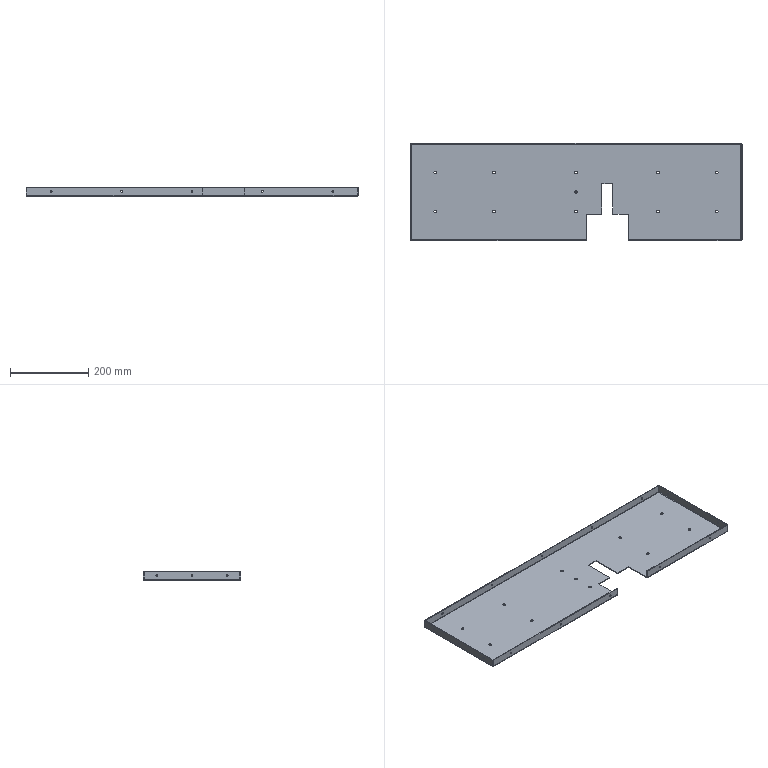Part | NX | features BREP 1 | 1 solid | 108 faces | box 849 x 249 x 22 mm | volume 481711 mm3 | cylinder 64 | plane 36 | spline 8 | commonest cylinder face diameters 4.5 x32 6.6 x22 2 x5 6 x5